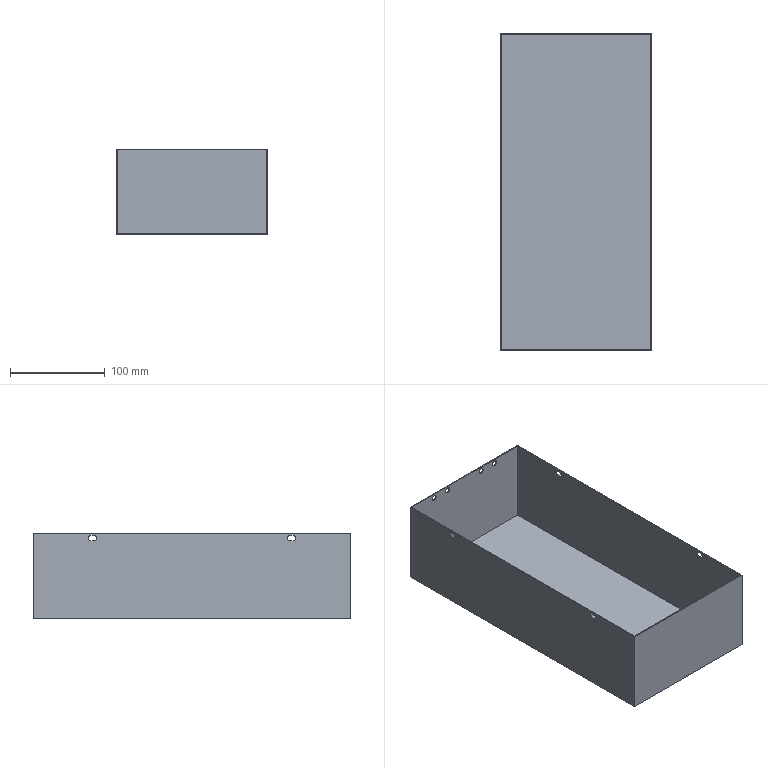Part | SolidWorks | features ICE 2, Extrusion 1, Shell 1 | 1 solid | 35 faces | box 160 x 335 x 90 mm | volume 168968 mm3 | plane 19 | cylinder 16 | commonest cylinder face diameters 5.6 x8 6 x8
STEP:
#1=CARTESIAN_POINT('',(-45.,166.3,88.));
#2=VERTEX_POINT('',#1);
#3=CARTESIAN_POINT('',(-45.,166.3,82.));
#4=VERTEX_POINT('',#3);
#5=CARTESIAN_POINT('',(-45.,166.3,85.));
#6=DIRECTION('',(0.,-1.,0.));
#7=DIRECTION('',(0.,0.,-1.));
#8=AXIS2_PLACEMENT_3D('',#5,#6,#7);
#9=CIRCLE('',#8,3.);
#10=EDGE_CURVE('',#2,#4,#9,.T.);
#11=ORIENTED_EDGE('',*,*,#10,.T.);
#12=CARTESIAN_POINT('',(-45.,167.5,82.));
#13=VERTEX_POINT('',#12);
#14=CARTESIAN_POINT('',(-45.,157.5,82.));
#15=DIRECTION('',(0.,1.,0.));
#16=VECTOR('',#15,1000.);
#17=LINE('',#14,#16);
#18=EDGE_CURVE('',#4,#13,#17,.T.);
#19=ORIENTED_EDGE('',*,*,#18,.T.);
#20=CARTESIAN_POINT('',(-45.,167.5,88.));
#21=VERTEX_POINT('',#20);
#22=CARTESIAN_POINT('',(-45.,167.5,85.));
#23=DIRECTION('',(0.,1.,0.));
#24=DIRECTION('',(0.,0.,1.));
#25=AXIS2_PLACEMENT_3D('',#22,#23,#24);
#26=CIRCLE('',#25,3.);
#27=EDGE_CURVE('',#13,#21,#26,.T.);
#28=ORIENTED_EDGE('',*,*,#27,.T.);
#29=CARTESIAN_POINT('',(-45.,157.5,88.));
#30=DIRECTION('',(0.,1.,0.));
#31=VECTOR('',#30,1000.);
#32=LINE('',#29,#31);
#33=EDGE_CURVE('',#2,#21,#32,.T.);
#34=ORIENTED_EDGE('',*,*,#33,.F.);
#35=EDGE_LOOP('',(#11,#19,#28,#34));
#36=FACE_OUTER_BOUND('',#35,.T.);
#37=CARTESIAN_POINT('',(-45.,157.5,85.));
#38=DIRECTION('',(0.,1.,0.));
#39=DIRECTION('',(0.,0.,1.));
#40=AXIS2_PLACEMENT_3D('',#37,#38,#39);
#41=CYLINDRICAL_SURFACE('',#40,3.);
#42=ADVANCED_FACE('',(#36),#41,.F.);
#43=CARTESIAN_POINT('',(-25.,166.3,88.));
#44=VERTEX_POINT('',#43);
#45=CARTESIAN_POINT('',(-25.,166.3,82.));
#46=VERTEX_POINT('',#45);
#47=CARTESIAN_POINT('',(-25.,166.3,85.));
#48=DIRECTION('',(0.,-1.,0.));
#49=DIRECTION('',(0.,0.,-1.));
#50=AXIS2_PLACEMENT_3D('',#47,#48,#49);
#51=CIRCLE('',#50,3.);
#52=EDGE_CURVE('',#44,#46,#51,.T.);
#53=ORIENTED_EDGE('',*,*,#52,.T.);
#54=CARTESIAN_POINT('',(-25.,167.5,82.));
#55=VERTEX_POINT('',#54);
#56=CARTESIAN_POINT('',(-25.,157.5,82.));
#57=DIRECTION('',(0.,1.,0.));
#58=VECTOR('',#57,1000.);
#59=LINE('',#56,#58);
#60=EDGE_CURVE('',#46,#55,#59,.T.);
#61=ORIENTED_EDGE('',*,*,#60,.T.);
#62=CARTESIAN_POINT('',(-25.,167.5,88.));
#63=VERTEX_POINT('',#62);
#64=CARTESIAN_POINT('',(-25.,167.5,85.));
#65=DIRECTION('',(0.,1.,0.));
#66=DIRECTION('',(0.,0.,1.));
#67=AXIS2_PLACEMENT_3D('',#64,#65,#66);
#68=CIRCLE('',#67,3.);
#69=EDGE_CURVE('',#55,#63,#68,.T.);
#70=ORIENTED_EDGE('',*,*,#69,.T.);
#71=CARTESIAN_POINT('',(-25.,157.5,88.));
#72=DIRECTION('',(0.,1.,0.));
#73=VECTOR('',#72,1000.);
#74=LINE('',#71,#73);
#75=EDGE_CURVE('',#44,#63,#74,.T.);
#76=ORIENTED_EDGE('',*,*,#75,.F.);
#77=EDGE_LOOP('',(#53,#61,#70,#76));
#78=FACE_OUTER_BOUND('',#77,.T.);
#79=CARTESIAN_POINT('',(-25.,157.5,85.));
#80=DIRECTION('',(0.,1.,0.));
#81=DIRECTION('',(0.,0.,1.));
#82=AXIS2_PLACEMENT_3D('',#79,#80,#81);
#83=CYLINDRICAL_SURFACE('',#82,3.);
#84=ADVANCED_FACE('',(#78),#83,.F.);
#85=CARTESIAN_POINT('',(25.,166.3,88.));
#86=VERTEX_POINT('',#85);
#87=CARTESIAN_POINT('',(25.,166.3,82.));
#88=VERTEX_POINT('',#87);
#89=CARTESIAN_POINT('',(25.,166.3,85.));
#90=DIRECTION('',(0.,-1.,0.));
#91=DIRECTION('',(0.,0.,-1.));
#92=AXIS2_PLACEMENT_3D('',#89,#90,#91);
#93=CIRCLE('',#92,3.);
#94=EDGE_CURVE('',#86,#88,#93,.T.);
#95=ORIENTED_EDGE('',*,*,#94,.T.);
#96=CARTESIAN_POINT('',(25.,167.5,82.));
#97=VERTEX_POINT('',#96);
#98=CARTESIAN_POINT('',(25.,157.5,82.));
#99=DIRECTION('',(0.,1.,0.));
#100=VECTOR('',#99,1000.);
#101=LINE('',#98,#100);
#102=EDGE_CURVE('',#88,#97,#101,.T.);
#103=ORIENTED_EDGE('',*,*,#102,.T.);
#104=CARTESIAN_POINT('',(25.,167.5,88.));
#105=VERTEX_POINT('',#104);
#106=CARTESIAN_POINT('',(25.,167.5,85.));
#107=DIRECTION('',(0.,1.,0.));
#108=DIRECTION('',(0.,0.,1.));
#109=AXIS2_PLACEMENT_3D('',#106,#107,#108);
#110=CIRCLE('',#109,3.);
#111=EDGE_CURVE('',#97,#105,#110,.T.);
#112=ORIENTED_EDGE('',*,*,#111,.T.);
#113=CARTESIAN_POINT('',(25.,157.5,88.));
#114=DIRECTION('',(0.,1.,0.));
#115=VECTOR('',#114,1000.);
#116=LINE('',#113,#115);
#117=EDGE_CURVE('',#86,#105,#116,.T.);
#118=ORIENTED_EDGE('',*,*,#117,.F.);
#119=EDGE_LOOP('',(#95,#103,#112,#118));
#120=FACE_OUTER_BOUND('',#119,.T.);
#121=CARTESIAN_POINT('',(25.,157.5,85.));
#122=DIRECTION('',(0.,1.,0.));
#123=DIRECTION('',(0.,0.,1.));
#124=AXIS2_PLACEMENT_3D('',#121,#122,#123);
#125=CYLINDRICAL_SURFACE('',#124,3.);
#126=ADVANCED_FACE('',(#120),#125,.F.);
#127=CARTESIAN_POINT('',(45.,166.3,88.));
#128=VERTEX_POINT('',#127);
#129=CARTESIAN_POINT('',(45.,166.3,82.));
#130=VERTEX_POINT('',#129);
#131=CARTESIAN_POINT('',(45.,166.3,85.));
#132=DIRECTION('',(0.,-1.,0.));
#133=DIRECTION('',(0.,0.,-1.));
#134=AXIS2_PLACEMENT_3D('',#131,#132,#133);
#135=CIRCLE('',#134,3.);
#136=EDGE_CURVE('',#128,#130,#135,.T.);
#137=ORIENTED_EDGE('',*,*,#136,.T.);
#138=CARTESIAN_POINT('',(45.,167.5,82.));
#139=VERTEX_POINT('',#138);
#140=CARTESIAN_POINT('',(45.,157.5,82.));
#141=DIRECTION('',(0.,1.,0.));
#142=VECTOR('',#141,1000.);
#143=LINE('',#140,#142);
#144=EDGE_CURVE('',#130,#139,#143,.T.);
#145=ORIENTED_EDGE('',*,*,#144,.T.);
#146=CARTESIAN_POINT('',(45.,167.5,88.));
#147=VERTEX_POINT('',#146);
#148=CARTESIAN_POINT('',(45.,167.5,85.));
#149=DIRECTION('',(0.,1.,0.));
#150=DIRECTION('',(0.,0.,1.));
#151=AXIS2_PLACEMENT_3D('',#148,#149,#150);
#152=CIRCLE('',#151,3.);
#153=EDGE_CURVE('',#139,#147,#152,.T.);
#154=ORIENTED_EDGE('',*,*,#153,.T.);
#155=CARTESIAN_POINT('',(45.,157.5,88.));
#156=DIRECTION('',(0.,1.,0.));
#157=VECTOR('',#156,1000.);
#158=LINE('',#155,#157);
#159=EDGE_CURVE('',#128,#147,#158,.T.);
#160=ORIENTED_EDGE('',*,*,#159,.F.);
#161=EDGE_LOOP('',(#137,#145,#154,#160));
#162=FACE_OUTER_BOUND('',#161,.T.);
#163=CARTESIAN_POINT('',(45.,157.5,85.));
#164=DIRECTION('',(0.,1.,0.));
#165=DIRECTION('',(0.,0.,1.));
#166=AXIS2_PLACEMENT_3D('',#163,#164,#165);
#167=CYLINDRICAL_SURFACE('',#166,3.);
#168=ADVANCED_FACE('',(#162),#167,.F.);
#169=CARTESIAN_POINT('',(80.,-167.5,90.));
#170=VERTEX_POINT('',#169);
#171=CARTESIAN_POINT('',(80.,167.5,90.));
#172=VERTEX_POINT('',#171);
#173=CARTESIAN_POINT('',(80.,-167.5,90.));
#174=DIRECTION('',(0.,1.,0.));
#175=VECTOR('',#174,1000.);
#176=LINE('',#173,#175);
#177=EDGE_CURVE('',#170,#172,#176,.T.);
#178=ORIENTED_EDGE('',*,*,#177,.T.);
#179=CARTESIAN_POINT('',(-80.,167.5,90.));
#180=VERTEX_POINT('',#179);
#181=CARTESIAN_POINT('',(-80.,167.5,90.));
#182=DIRECTION('',(-1.,0.,0.));
#183=VECTOR('',#182,1000.);
#184=LINE('',#181,#183);
#185=EDGE_CURVE('',#172,#180,#184,.T.);
#186=ORIENTED_EDGE('',*,*,#185,.T.);
#187=CARTESIAN_POINT('',(-80.,-167.5,90.));
#188=VERTEX_POINT('',#187);
#189=CARTESIAN_POINT('',(-80.,-167.5,90.));
#190=DIRECTION('',(0.,-1.,0.));
#191=VECTOR('',#190,1000.);
#192=LINE('',#189,#191);
#193=EDGE_CURVE('',#180,#188,#192,.T.);
#194=ORIENTED_EDGE('',*,*,#193,.T.);
#195=CARTESIAN_POINT('',(-80.,-167.5,90.));
#196=DIRECTION('',(1.,0.,0.));
#197=VECTOR('',#196,1000.);
#198=LINE('',#195,#197);
#199=EDGE_CURVE('',#188,#170,#198,.T.);
#200=ORIENTED_EDGE('',*,*,#199,.T.);
#201=EDGE_LOOP('',(#178,#186,#194,#200));
#202=FACE_OUTER_BOUND('',#201,.T.);
#203=CARTESIAN_POINT('',(78.8,-166.3,90.));
#204=VERTEX_POINT('',#203);
#205=CARTESIAN_POINT('',(78.8,166.3,90.));
#206=VERTEX_POINT('',#205);
#207=CARTESIAN_POINT('',(78.8,0.,90.));
#208=DIRECTION('',(0.,1.,0.));
#209=VECTOR('',#208,1000.);
#210=LINE('',#207,#209);
#211=EDGE_CURVE('',#204,#206,#210,.T.);
#212=ORIENTED_EDGE('',*,*,#211,.F.);
#213=CARTESIAN_POINT('',(-78.8,-166.3,90.));
#214=VERTEX_POINT('',#213);
#215=CARTESIAN_POINT('',(0.,-166.3,90.));
#216=DIRECTION('',(1.,0.,0.));
#217=VECTOR('',#216,1000.);
#218=LINE('',#215,#217);
#219=EDGE_CURVE('',#214,#204,#218,.T.);
#220=ORIENTED_EDGE('',*,*,#219,.F.);
#221=CARTESIAN_POINT('',(-78.8,166.3,90.));
#222=VERTEX_POINT('',#221);
#223=CARTESIAN_POINT('',(-78.8,0.,90.));
#224=DIRECTION('',(0.,-1.,0.));
#225=VECTOR('',#224,1000.);
#226=LINE('',#223,#225);
#227=EDGE_CURVE('',#222,#214,#226,.T.);
#228=ORIENTED_EDGE('',*,*,#227,.F.);
#229=CARTESIAN_POINT('',(0.,166.3,90.));
#230=DIRECTION('',(-1.,0.,0.));
#231=VECTOR('',#230,1000.);
#232=LINE('',#229,#231);
#233=EDGE_CURVE('',#206,#222,#232,.T.);
#234=ORIENTED_EDGE('',*,*,#233,.F.);
#235=EDGE_LOOP('',(#212,#220,#228,#234));
#236=FACE_BOUND('',#235,.T.);
#237=CARTESIAN_POINT('',(0.,0.,90.));
#238=DIRECTION('',(0.,0.,-1.));
#239=DIRECTION('',(-1.,0.,0.));
#240=AXIS2_PLACEMENT_3D('',#237,#238,#239);
#241=PLANE('',#240);
#242=ADVANCED_FACE('',(#202,#236),#241,.F.);
#243=CARTESIAN_POINT('',(80.,103.5,87.8));
#244=VERTEX_POINT('',#243);
#245=CARTESIAN_POINT('',(80.,106.5,87.8));
#246=VERTEX_POINT('',#245);
#247=CARTESIAN_POINT('',(80.,106.5,87.8));
#248=DIRECTION('',(0.,1.,0.));
#249=VECTOR('',#248,1000.);
#250=LINE('',#247,#249);
#251=EDGE_CURVE('',#244,#246,#250,.T.);
#252=ORIENTED_EDGE('',*,*,#251,.T.);
#253=CARTESIAN_POINT('',(80.,106.5,82.2));
#254=VERTEX_POINT('',#253);
#255=CARTESIAN_POINT('',(80.,106.5,85.));
#256=DIRECTION('',(-1.,0.,0.));
#257=DIRECTION('',(0.,0.,1.));
#258=AXIS2_PLACEMENT_3D('',#255,#256,#257);
#259=CIRCLE('',#258,2.8);
#260=EDGE_CURVE('',#246,#254,#259,.T.);
#261=ORIENTED_EDGE('',*,*,#260,.T.);
#262=CARTESIAN_POINT('',(80.,103.5,82.2));
#263=VERTEX_POINT('',#262);
#264=CARTESIAN_POINT('',(80.,106.5,82.2));
#265=DIRECTION('',(0.,-1.,0.));
#266=VECTOR('',#265,1000.);
#267=LINE('',#264,#266);
#268=EDGE_CURVE('',#254,#263,#267,.T.);
#269=ORIENTED_EDGE('',*,*,#268,.T.);
#270=CARTESIAN_POINT('',(80.,103.5,85.));
#271=DIRECTION('',(-1.,0.,0.));
#272=DIRECTION('',(0.,0.,1.));
#273=AXIS2_PLACEMENT_3D('',#270,#271,#272);
#274=CIRCLE('',#273,2.8);
#275=EDGE_CURVE('',#263,#244,#274,.T.);
#276=ORIENTED_EDGE('',*,*,#275,.T.);
#277=EDGE_LOOP('',(#252,#261,#269,#276));
#278=FACE_BOUND('',#277,.T.);
#279=CARTESIAN_POINT('',(80.,-103.5,82.2));
#280=VERTEX_POINT('',#279);
#281=CARTESIAN_POINT('',(80.,-106.5,82.2));
#282=VERTEX_POINT('',#281);
#283=CARTESIAN_POINT('',(80.,-106.5,82.2));
#284=DIRECTION('',(0.,-1.,0.));
#285=VECTOR('',#284,1000.);
#286=LINE('',#283,#285);
#287=EDGE_CURVE('',#280,#282,#286,.T.);
#288=ORIENTED_EDGE('',*,*,#287,.T.);
#289=CARTESIAN_POINT('',(80.,-106.5,87.8));
#290=VERTEX_POINT('',#289);
#291=CARTESIAN_POINT('',(80.,-106.5,85.));
#292=DIRECTION('',(-1.,0.,0.));
#293=DIRECTION('',(0.,0.,-1.));
#294=AXIS2_PLACEMENT_3D('',#291,#292,#293);
#295=CIRCLE('',#294,2.8);
#296=EDGE_CURVE('',#282,#290,#295,.T.);
#297=ORIENTED_EDGE('',*,*,#296,.T.);
#298=CARTESIAN_POINT('',(80.,-103.5,87.8));
#299=VERTEX_POINT('',#298);
#300=CARTESIAN_POINT('',(80.,-106.5,87.8));
#301=DIRECTION('',(0.,1.,0.));
#302=VECTOR('',#301,1000.);
#303=LINE('',#300,#302);
#304=EDGE_CURVE('',#290,#299,#303,.T.);
#305=ORIENTED_EDGE('',*,*,#304,.T.);
#306=CARTESIAN_POINT('',(80.,-103.5,85.));
#307=DIRECTION('',(-1.,0.,0.));
#308=DIRECTION('',(0.,0.,-1.));
#309=AXIS2_PLACEMENT_3D('',#306,#307,#308);
#310=CIRCLE('',#309,2.8);
#311=EDGE_CURVE('',#299,#280,#310,.T.);
#312=ORIENTED_EDGE('',*,*,#311,.T.);
#313=EDGE_LOOP('',(#288,#297,#305,#312));
#314=FACE_BOUND('',#313,.T.);
#315=CARTESIAN_POINT('',(80.,-167.5,0.));
#316=VERTEX_POINT('',#315);
#317=CARTESIAN_POINT('',(80.,167.5,0.));
#318=VERTEX_POINT('',#317);
#319=CARTESIAN_POINT('',(80.,-167.5,0.));
#320=DIRECTION('',(0.,1.,0.));
#321=VECTOR('',#320,1000.);
#322=LINE('',#319,#321);
#323=EDGE_CURVE('',#316,#318,#322,.T.);
#324=ORIENTED_EDGE('',*,*,#323,.T.);
#325=CARTESIAN_POINT('',(80.,167.5,90.));
#326=DIRECTION('',(0.,0.,-1.));
#327=VECTOR('',#326,1000.);
#328=LINE('',#325,#327);
#329=EDGE_CURVE('',#172,#318,#328,.T.);
#330=ORIENTED_EDGE('',*,*,#329,.F.);
#331=ORIENTED_EDGE('',*,*,#177,.F.);
#332=CARTESIAN_POINT('',(80.,-167.5,90.));
#333=DIRECTION('',(0.,0.,-1.));
#334=VECTOR('',#333,1000.);
#335=LINE('',#332,#334);
#336=EDGE_CURVE('',#170,#316,#335,.T.);
#337=ORIENTED_EDGE('',*,*,#336,.T.);
#338=EDGE_LOOP('',(#324,#330,#331,#337));
#339=FACE_OUTER_BOUND('',#338,.T.);
#340=CARTESIAN_POINT('',(80.,-167.5,90.));
#341=DIRECTION('',(-1.,0.,0.));
#342=DIRECTION('',(0.,0.,1.));
#343=AXIS2_PLACEMENT_3D('',#340,#341,#342);
#344=PLANE('',#343);
#345=ADVANCED_FACE('',(#278,#314,#339),#344,.F.);
#346=CARTESIAN_POINT('',(-45.,167.5,85.));
#347=DIRECTION('',(0.,1.,0.));
#348=DIRECTION('',(0.,0.,1.));
#349=AXIS2_PLACEMENT_3D('',#346,#347,#348);
#350=CIRCLE('',#349,3.);
#351=EDGE_CURVE('',#21,#13,#350,.T.);
#352=ORIENTED_EDGE('',*,*,#351,.F.);
#353=ORIENTED_EDGE('',*,*,#27,.F.);
#354=EDGE_LOOP('',(#352,#353));
#355=FACE_BOUND('',#354,.T.);
#356=CARTESIAN_POINT('',(-25.,167.5,85.));
#357=DIRECTION('',(0.,1.,0.));
#358=DIRECTION('',(0.,0.,1.));
#359=AXIS2_PLACEMENT_3D('',#356,#357,#358);
#360=CIRCLE('',#359,3.);
#361=EDGE_CURVE('',#63,#55,#360,.T.);
#362=ORIENTED_EDGE('',*,*,#361,.F.);
#363=ORIENTED_EDGE('',*,*,#69,.F.);
#364=EDGE_LOOP('',(#362,#363));
#365=FACE_BOUND('',#364,.T.);
#366=CARTESIAN_POINT('',(25.,167.5,85.));
#367=DIRECTION('',(0.,1.,0.));
#368=DIRECTION('',(0.,0.,1.));
#369=AXIS2_PLACEMENT_3D('',#366,#367,#368);
#370=CIRCLE('',#369,3.);
#371=EDGE_CURVE('',#105,#97,#370,.T.);
#372=ORIENTED_EDGE('',*,*,#371,.F.);
#373=ORIENTED_EDGE('',*,*,#111,.F.);
#374=EDGE_LOOP('',(#372,#373));
#375=FACE_BOUND('',#374,.T.);
#376=CARTESIAN_POINT('',(45.,167.5,85.));
#377=DIRECTION('',(0.,1.,0.));
#378=DIRECTION('',(0.,0.,1.));
#379=AXIS2_PLACEMENT_3D('',#376,#377,#378);
#380=CIRCLE('',#379,3.);
#381=EDGE_CURVE('',#147,#139,#380,.T.);
#382=ORIENTED_EDGE('',*,*,#381,.F.);
#383=ORIENTED_EDGE('',*,*,#153,.F.);
#384=EDGE_LOOP('',(#382,#383));
#385=FACE_BOUND('',#384,.T.);
#386=CARTESIAN_POINT('',(-80.,167.5,0.));
#387=VERTEX_POINT('',#386);
#388=CARTESIAN_POINT('',(-80.,167.5,0.));
#389=DIRECTION('',(-1.,0.,0.));
#390=VECTOR('',#389,1000.);
#391=LINE('',#388,#390);
#392=EDGE_CURVE('',#318,#387,#391,.T.);
#393=ORIENTED_EDGE('',*,*,#392,.T.);
#394=CARTESIAN_POINT('',(-80.,167.5,90.));
#395=DIRECTION('',(0.,0.,-1.));
#396=VECTOR('',#395,1000.);
#397=LINE('',#394,#396);
#398=EDGE_CURVE('',#180,#387,#397,.T.);
#399=ORIENTED_EDGE('',*,*,#398,.F.);
#400=ORIENTED_EDGE('',*,*,#185,.F.);
#401=ORIENTED_EDGE('',*,*,#329,.T.);
#402=EDGE_LOOP('',(#393,#399,#400,#401));
#403=FACE_OUTER_BOUND('',#402,.T.);
#404=CARTESIAN_POINT('',(-80.,167.5,90.));
#405=DIRECTION('',(0.,-1.,0.));
#406=DIRECTION('',(0.,0.,-1.));
#407=AXIS2_PLACEMENT_3D('',#404,#405,#406);
#408=PLANE('',#407);
#409=ADVANCED_FACE('',(#355,#365,#375,#385,#403),#408,.F.);
#410=CARTESIAN_POINT('',(-80.,106.5,82.2));
#411=VERTEX_POINT('',#410);
#412=CARTESIAN_POINT('',(-80.,103.5,82.2));
#413=VERTEX_POINT('',#412);
#414=CARTESIAN_POINT('',(-80.,106.5,82.2));
#415=DIRECTION('',(0.,-1.,0.));
#416=VECTOR('',#415,1000.);
#417=LINE('',#414,#416);
#418=EDGE_CURVE('',#411,#413,#417,.T.);
#419=ORIENTED_EDGE('',*,*,#418,.F.);
#420=CARTESIAN_POINT('',(-80.,106.5,87.8));
#421=VERTEX_POINT('',#420);
#422=CARTESIAN_POINT('',(-80.,106.5,85.));
#423=DIRECTION('',(-1.,0.,0.));
#424=DIRECTION('',(0.,0.,1.));
#425=AXIS2_PLACEMENT_3D('',#422,#423,#424);
#426=CIRCLE('',#425,2.8);
#427=EDGE_CURVE('',#421,#411,#426,.T.);
#428=ORIENTED_EDGE('',*,*,#427,.F.);
#429=CARTESIAN_POINT('',(-80.,103.5,87.8));
#430=VERTEX_POINT('',#429);
#431=CARTESIAN_POINT('',(-80.,106.5,87.8));
#432=DIRECTION('',(0.,1.,0.));
#433=VECTOR('',#432,1000.);
#434=LINE('',#431,#433);
#435=EDGE_CURVE('',#430,#421,#434,.T.);
#436=ORIENTED_EDGE('',*,*,#435,.F.);
#437=CARTESIAN_POINT('',(-80.,103.5,85.));
#438=DIRECTION('',(-1.,0.,0.));
#439=DIRECTION('',(0.,0.,1.));
#440=AXIS2_PLACEMENT_3D('',#437,#438,#439);
#441=CIRCLE('',#440,2.8);
#442=EDGE_CURVE('',#413,#430,#441,.T.);
#443=ORIENTED_EDGE('',*,*,#442,.F.);
#444=EDGE_LOOP('',(#419,#428,#436,#443));
#445=FACE_BOUND('',#444,.T.);
#446=CARTESIAN_POINT('',(-80.,-106.5,87.8));
#447=VERTEX_POINT('',#446);
#448=CARTESIAN_POINT('',(-80.,-103.5,87.8));
#449=VERTEX_POINT('',#448);
#450=CARTESIAN_POINT('',(-80.,-106.5,87.8));
#451=DIRECTION('',(0.,1.,0.));
#452=VECTOR('',#451,1000.);
#453=LINE('',#450,#452);
#454=EDGE_CURVE('',#447,#449,#453,.T.);
#455=ORIENTED_EDGE('',*,*,#454,.F.);
#456=CARTESIAN_POINT('',(-80.,-106.5,82.2));
#457=VERTEX_POINT('',#456);
#458=CARTESIAN_POINT('',(-80.,-106.5,85.));
#459=DIRECTION('',(-1.,0.,0.));
#460=DIRECTION('',(0.,0.,-1.));
#461=AXIS2_PLACEMENT_3D('',#458,#459,#460);
#462=CIRCLE('',#461,2.8);
#463=EDGE_CURVE('',#457,#447,#462,.T.);
#464=ORIENTED_EDGE('',*,*,#463,.F.);
#465=CARTESIAN_POINT('',(-80.,-103.5,82.2));
#466=VERTEX_POINT('',#465);
#467=CARTESIAN_POINT('',(-80.,-106.5,82.2));
#468=DIRECTION('',(0.,-1.,0.));
#469=VECTOR('',#468,1000.);
#470=LINE('',#467,#469);
#471=EDGE_CURVE('',#466,#457,#470,.T.);
#472=ORIENTED_EDGE('',*,*,#471,.F.);
#473=CARTESIAN_POINT('',(-80.,-103.5,85.));
#474=DIRECTION('',(-1.,0.,0.));
#475=DIRECTION('',(0.,0.,-1.));
#476=AXIS2_PLACEMENT_3D('',#473,#474,#475);
#477=CIRCLE('',#476,2.8);
#478=EDGE_CURVE('',#449,#466,#477,.T.);
#479=ORIENTED_EDGE('',*,*,#478,.F.);
#480=EDGE_LOOP('',(#455,#464,#472,#479));
#481=FACE_BOUND('',#480,.T.);
#482=CARTESIAN_POINT('',(-80.,-167.5,0.));
#483=VERTEX_POINT('',#482);
#484=CARTESIAN_POINT('',(-80.,-167.5,0.));
#485=DIRECTION('',(0.,-1.,0.));
#486=VECTOR('',#485,1000.);
#487=LINE('',#484,#486);
#488=EDGE_CURVE('',#387,#483,#487,.T.);
#489=ORIENTED_EDGE('',*,*,#488,.T.);
#490=CARTESIAN_POINT('',(-80.,-167.5,90.));
#491=DIRECTION('',(0.,0.,-1.));
#492=VECTOR('',#491,1000.);
#493=LINE('',#490,#492);
#494=EDGE_CURVE('',#188,#483,#493,.T.);
#495=ORIENTED_EDGE('',*,*,#494,.F.);
#496=ORIENTED_EDGE('',*,*,#193,.F.);
#497=ORIENTED_EDGE('',*,*,#398,.T.);
#498=EDGE_LOOP('',(#489,#495,#496,#497));
#499=FACE_OUTER_BOUND('',#498,.T.);
#500=CARTESIAN_POINT('',(-80.,-167.5,90.));
#501=DIRECTION('',(1.,0.,0.));
#502=DIRECTION('',(0.,0.,-1.));
#503=AXIS2_PLACEMENT_3D('',#500,#501,#502);
#504=PLANE('',#503);
#505=ADVANCED_FACE('',(#445,#481,#499),#504,.F.);
#506=CARTESIAN_POINT('',(-80.,-167.5,0.));
#507=DIRECTION('',(1.,0.,0.));
#508=VECTOR('',#507,1000.);
#509=LINE('',#506,#508);
#510=EDGE_CURVE('',#483,#316,#509,.T.);
#511=ORIENTED_EDGE('',*,*,#510,.T.);
#512=ORIENTED_EDGE('',*,*,#336,.F.);
#513=ORIENTED_EDGE('',*,*,#199,.F.);
#514=ORIENTED_EDGE('',*,*,#494,.T.);
#515=EDGE_LOOP('',(#511,#512,#513,#514));
#516=FACE_OUTER_BOUND('',#515,.T.);
#517=CARTESIAN_POINT('',(-80.,-167.5,90.));
#518=DIRECTION('',(0.,1.,0.));
#519=DIRECTION('',(0.,0.,1.));
#520=AXIS2_PLACEMENT_3D('',#517,#518,#519);
#521=PLANE('',#520);
#522=ADVANCED_FACE('',(#516),#521,.F.);
#523=ORIENTED_EDGE('',*,*,#323,.F.);
#524=ORIENTED_EDGE('',*,*,#510,.F.);
#525=ORIENTED_EDGE('',*,*,#488,.F.);
#526=ORIENTED_EDGE('',*,*,#392,.F.);
#527=EDGE_LOOP('',(#523,#524,#525,#526));
#528=FACE_OUTER_BOUND('',#527,.T.);
#529=CARTESIAN_POINT('',(0.,0.,0.));
#530=DIRECTION('',(0.,0.,-1.));
#531=DIRECTION('',(-1.,0.,0.));
#532=AXIS2_PLACEMENT_3D('',#529,#530,#531);
#533=PLANE('',#532);
#534=ADVANCED_FACE('',(#528),#533,.T.);
#535=CARTESIAN_POINT('',(78.8,106.5,87.8));
#536=VERTEX_POINT('',#535);
#537=CARTESIAN_POINT('',(78.8,106.5,82.2));
#538=VERTEX_POINT('',#537);
#539=CARTESIAN_POINT('',(78.8,106.5,85.));
#540=DIRECTION('',(-1.,0.,0.));
#541=DIRECTION('',(0.,0.,1.));
#542=AXIS2_PLACEMENT_3D('',#539,#540,#541);
#543=CIRCLE('',#542,2.8);
#544=EDGE_CURVE('',#536,#538,#543,.T.);
#545=ORIENTED_EDGE('',*,*,#544,.F.);
#546=CARTESIAN_POINT('',(78.8,103.5,87.8));
#547=VERTEX_POINT('',#546);
#548=CARTESIAN_POINT('',(78.8,-167.5,87.8));
#549=DIRECTION('',(0.,1.,0.));
#550=VECTOR('',#549,1000.);
#551=LINE('',#548,#550);
#552=EDGE_CURVE('',#547,#536,#551,.T.);
#553=ORIENTED_EDGE('',*,*,#552,.F.);
#554=CARTESIAN_POINT('',(78.8,103.5,82.2));
#555=VERTEX_POINT('',#554);
#556=CARTESIAN_POINT('',(78.8,103.5,85.));
#557=DIRECTION('',(-1.,0.,0.));
#558=DIRECTION('',(0.,0.,1.));
#559=AXIS2_PLACEMENT_3D('',#556,#557,#558);
#560=CIRCLE('',#559,2.8);
#561=EDGE_CURVE('',#555,#547,#560,.T.);
#562=ORIENTED_EDGE('',*,*,#561,.F.);
#563=CARTESIAN_POINT('',(78.8,-167.5,82.2));
#564=DIRECTION('',(0.,-1.,0.));
#565=VECTOR('',#564,1000.);
#566=LINE('',#563,#565);
#567=EDGE_CURVE('',#538,#555,#566,.T.);
#568=ORIENTED_EDGE('',*,*,#567,.F.);
#569=EDGE_LOOP('',(#545,#553,#562,#568));
#570=FACE_BOUND('',#569,.T.);
#571=CARTESIAN_POINT('',(78.8,-106.5,82.2));
#572=VERTEX_POINT('',#571);
#573=CARTESIAN_POINT('',(78.8,-106.5,87.8));
#574=VERTEX_POINT('',#573);
#575=CARTESIAN_POINT('',(78.8,-106.5,85.));
#576=DIRECTION('',(-1.,0.,0.));
#577=DIRECTION('',(0.,0.,1.));
#578=AXIS2_PLACEMENT_3D('',#575,#576,#577);
#579=CIRCLE('',#578,2.8);
#580=EDGE_CURVE('',#572,#574,#579,.T.);
#581=ORIENTED_EDGE('',*,*,#580,.F.);
#582=CARTESIAN_POINT('',(78.8,-103.5,82.2));
#583=VERTEX_POINT('',#582);
#584=CARTESIAN_POINT('',(78.8,-167.5,82.2));
#585=DIRECTION('',(0.,-1.,0.));
#586=VECTOR('',#585,1000.);
#587=LINE('',#584,#586);
#588=EDGE_CURVE('',#583,#572,#587,.T.);
#589=ORIENTED_EDGE('',*,*,#588,.F.);
#590=CARTESIAN_POINT('',(78.8,-103.5,87.8));
#591=VERTEX_POINT('',#590);
#592=CARTESIAN_POINT('',(78.8,-103.5,85.));
#593=DIRECTION('',(-1.,0.,0.));
#594=DIRECTION('',(0.,0.,1.));
#595=AXIS2_PLACEMENT_3D('',#592,#593,#594);
#596=CIRCLE('',#595,2.8);
#597=EDGE_CURVE('',#591,#583,#596,.T.);
#598=ORIENTED_EDGE('',*,*,#597,.F.);
#599=CARTESIAN_POINT('',(78.8,-167.5,87.8));
#600=DIRECTION('',(0.,1.,0.));
#601=VECTOR('',#600,1000.);
#602=LINE('',#599,#601);
#603=EDGE_CURVE('',#574,#591,#602,.T.);
#604=ORIENTED_EDGE('',*,*,#603,.F.);
#605=EDGE_LOOP('',(#581,#589,#598,#604));
#606=FACE_BOUND('',#605,.T.);
#607=CARTESIAN_POINT('',(78.8,-166.3,1.2));
#608=VERTEX_POINT('',#607);
#609=CARTESIAN_POINT('',(78.8,166.3,1.2));
#610=VERTEX_POINT('',#609);
#611=CARTESIAN_POINT('',(78.8,0.,1.2));
#612=DIRECTION('',(0.,1.,0.));
#613=VECTOR('',#612,1000.);
#614=LINE('',#611,#613);
#615=EDGE_CURVE('',#608,#610,#614,.T.);
#616=ORIENTED_EDGE('',*,*,#615,.F.);
#617=CARTESIAN_POINT('',(78.8,-166.3,90.));
#618=DIRECTION('',(0.,0.,-1.));
#619=VECTOR('',#618,1000.);
#620=LINE('',#617,#619);
#621=EDGE_CURVE('',#204,#608,#620,.T.);
#622=ORIENTED_EDGE('',*,*,#621,.F.);
#623=ORIENTED_EDGE('',*,*,#211,.T.);
#624=CARTESIAN_POINT('',(78.8,166.3,90.));
#625=DIRECTION('',(0.,0.,-1.));
#626=VECTOR('',#625,1000.);
#627=LINE('',#624,#626);
#628=EDGE_CURVE('',#206,#610,#627,.T.);
#629=ORIENTED_EDGE('',*,*,#628,.T.);
#630=EDGE_LOOP('',(#616,#622,#623,#629));
#631=FACE_OUTER_BOUND('',#630,.T.);
#632=CARTESIAN_POINT('',(78.8,-167.5,90.));
#633=DIRECTION('',(-1.,0.,0.));
#634=DIRECTION('',(0.,0.,1.));
#635=AXIS2_PLACEMENT_3D('',#632,#633,#634);
#636=PLANE('',#635);
#637=ADVANCED_FACE('',(#570,#606,#631),#636,.T.);
#638=ORIENTED_EDGE('',*,*,#10,.F.);
#639=CARTESIAN_POINT('',(-45.,166.3,85.));
#640=DIRECTION('',(0.,-1.,0.));
#641=DIRECTION('',(0.,0.,-1.));
#642=AXIS2_PLACEMENT_3D('',#639,#640,#641);
#643=CIRCLE('',#642,3.);
#644=EDGE_CURVE('',#4,#2,#643,.T.);
#645=ORIENTED_EDGE('',*,*,#644,.F.);
#646=EDGE_LOOP('',(#638,#645));
#647=FACE_BOUND('',#646,.T.);
#648=ORIENTED_EDGE('',*,*,#52,.F.);
#649=CARTESIAN_POINT('',(-25.,166.3,85.));
#650=DIRECTION('',(0.,-1.,0.));
#651=DIRECTION('',(0.,0.,-1.));
#652=AXIS2_PLACEMENT_3D('',#649,#650,#651);
#653=CIRCLE('',#652,3.);
#654=EDGE_CURVE('',#46,#44,#653,.T.);
#655=ORIENTED_EDGE('',*,*,#654,.F.);
#656=EDGE_LOOP('',(#648,#655));
#657=FACE_BOUND('',#656,.T.);
#658=ORIENTED_EDGE('',*,*,#94,.F.);
#659=CARTESIAN_POINT('',(25.,166.3,85.));
#660=DIRECTION('',(0.,-1.,0.));
#661=DIRECTION('',(0.,0.,-1.));
#662=AXIS2_PLACEMENT_3D('',#659,#660,#661);
#663=CIRCLE('',#662,3.);
#664=EDGE_CURVE('',#88,#86,#663,.T.);
#665=ORIENTED_EDGE('',*,*,#664,.F.);
#666=EDGE_LOOP('',(#658,#665));
#667=FACE_BOUND('',#666,.T.);
#668=ORIENTED_EDGE('',*,*,#136,.F.);
#669=CARTESIAN_POINT('',(45.,166.3,85.));
#670=DIRECTION('',(0.,-1.,0.));
#671=DIRECTION('',(0.,0.,-1.));
#672=AXIS2_PLACEMENT_3D('',#669,#670,#671);
#673=CIRCLE('',#672,3.);
#674=EDGE_CURVE('',#130,#128,#673,.T.);
#675=ORIENTED_EDGE('',*,*,#674,.F.);
#676=EDGE_LOOP('',(#668,#675));
#677=FACE_BOUND('',#676,.T.);
#678=CARTESIAN_POINT('',(-78.8,166.3,1.2));
#679=VERTEX_POINT('',#678);
#680=CARTESIAN_POINT('',(0.,166.3,1.2));
#681=DIRECTION('',(-1.,0.,0.));
#682=VECTOR('',#681,1000.);
#683=LINE('',#680,#682);
#684=EDGE_CURVE('',#610,#679,#683,.T.);
#685=ORIENTED_EDGE('',*,*,#684,.F.);
#686=ORIENTED_EDGE('',*,*,#628,.F.);
#687=ORIENTED_EDGE('',*,*,#233,.T.);
#688=CARTESIAN_POINT('',(-78.8,166.3,90.));
#689=DIRECTION('',(0.,0.,-1.));
#690=VECTOR('',#689,1000.);
#691=LINE('',#688,#690);
#692=EDGE_CURVE('',#222,#679,#691,.T.);
#693=ORIENTED_EDGE('',*,*,#692,.T.);
#694=EDGE_LOOP('',(#685,#686,#687,#693));
#695=FACE_OUTER_BOUND('',#694,.T.);
#696=CARTESIAN_POINT('',(-80.,166.3,90.));
#697=DIRECTION('',(0.,-1.,0.));
#698=DIRECTION('',(0.,0.,-1.));
#699=AXIS2_PLACEMENT_3D('',#696,#697,#698);
#700=PLANE('',#699);
#701=ADVANCED_FACE('',(#647,#657,#667,#677,#695),#700,.T.);
#702=CARTESIAN_POINT('',(-78.8,106.5,82.2));
#703=VERTEX_POINT('',#702);
#704=CARTESIAN_POINT('',(-78.8,106.5,87.8));
#705=VERTEX_POINT('',#704);
#706=CARTESIAN_POINT('',(-78.8,106.5,85.));
#707=DIRECTION('',(1.,0.,0.));
#708=DIRECTION('',(0.,0.,-1.));
#709=AXIS2_PLACEMENT_3D('',#706,#707,#708);
#710=CIRCLE('',#709,2.8);
#711=EDGE_CURVE('',#703,#705,#710,.T.);
#712=ORIENTED_EDGE('',*,*,#711,.F.);
#713=CARTESIAN_POINT('',(-78.8,103.5,82.2));
#714=VERTEX_POINT('',#713);
#715=CARTESIAN_POINT('',(-78.8,-167.5,82.2));
#716=DIRECTION('',(0.,1.,0.));
#717=VECTOR('',#716,1000.);
#718=LINE('',#715,#717);
#719=EDGE_CURVE('',#714,#703,#718,.T.);
#720=ORIENTED_EDGE('',*,*,#719,.F.);
#721=CARTESIAN_POINT('',(-78.8,103.5,87.8));
#722=VERTEX_POINT('',#721);
#723=CARTESIAN_POINT('',(-78.8,103.5,85.));
#724=DIRECTION('',(1.,0.,0.));
#725=DIRECTION('',(0.,0.,-1.));
#726=AXIS2_PLACEMENT_3D('',#723,#724,#725);
#727=CIRCLE('',#726,2.8);
#728=EDGE_CURVE('',#722,#714,#727,.T.);
#729=ORIENTED_EDGE('',*,*,#728,.F.);
#730=CARTESIAN_POINT('',(-78.8,-167.5,87.8));
#731=DIRECTION('',(0.,-1.,0.));
#732=VECTOR('',#731,1000.);
#733=LINE('',#730,#732);
#734=EDGE_CURVE('',#705,#722,#733,.T.);
#735=ORIENTED_EDGE('',*,*,#734,.F.);
#736=EDGE_LOOP('',(#712,#720,#729,#735));
#737=FACE_BOUND('',#736,.T.);
#738=CARTESIAN_POINT('',(-78.8,-106.5,87.8));
#739=VERTEX_POINT('',#738);
#740=CARTESIAN_POINT('',(-78.8,-106.5,82.2));
#741=VERTEX_POINT('',#740);
#742=CARTESIAN_POINT('',(-78.8,-106.5,85.));
#743=DIRECTION('',(1.,0.,0.));
#744=DIRECTION('',(0.,0.,-1.));
#745=AXIS2_PLACEMENT_3D('',#742,#743,#744);
#746=CIRCLE('',#745,2.8);
#747=EDGE_CURVE('',#739,#741,#746,.T.);
#748=ORIENTED_EDGE('',*,*,#747,.F.);
#749=CARTESIAN_POINT('',(-78.8,-103.5,87.8));
#750=VERTEX_POINT('',#749);
#751=CARTESIAN_POINT('',(-78.8,-167.5,87.8));
#752=DIRECTION('',(0.,-1.,0.));
#753=VECTOR('',#752,1000.);
#754=LINE('',#751,#753);
#755=EDGE_CURVE('',#750,#739,#754,.T.);
#756=ORIENTED_EDGE('',*,*,#755,.F.);
#757=CARTESIAN_POINT('',(-78.8,-103.5,82.2));
#758=VERTEX_POINT('',#757);
#759=CARTESIAN_POINT('',(-78.8,-103.5,85.));
#760=DIRECTION('',(1.,0.,0.));
#761=DIRECTION('',(0.,0.,-1.));
#762=AXIS2_PLACEMENT_3D('',#759,#760,#761);
#763=CIRCLE('',#762,2.8);
#764=EDGE_CURVE('',#758,#750,#763,.T.);
#765=ORIENTED_EDGE('',*,*,#764,.F.);
#766=CARTESIAN_POINT('',(-78.8,-167.5,82.2));
#767=DIRECTION('',(0.,1.,0.));
#768=VECTOR('',#767,1000.);
#769=LINE('',#766,#768);
#770=EDGE_CURVE('',#741,#758,#769,.T.);
#771=ORIENTED_EDGE('',*,*,#770,.F.);
#772=EDGE_LOOP('',(#748,#756,#765,#771));
#773=FACE_BOUND('',#772,.T.);
#774=CARTESIAN_POINT('',(-78.8,-166.3,1.2));
#775=VERTEX_POINT('',#774);
#776=CARTESIAN_POINT('',(-78.8,0.,1.2));
#777=DIRECTION('',(0.,-1.,0.));
#778=VECTOR('',#777,1000.);
#779=LINE('',#776,#778);
#780=EDGE_CURVE('',#679,#775,#779,.T.);
#781=ORIENTED_EDGE('',*,*,#780,.F.);
#782=ORIENTED_EDGE('',*,*,#692,.F.);
#783=ORIENTED_EDGE('',*,*,#227,.T.);
#784=CARTESIAN_POINT('',(-78.8,-166.3,90.));
#785=DIRECTION('',(0.,0.,-1.));
#786=VECTOR('',#785,1000.);
#787=LINE('',#784,#786);
#788=EDGE_CURVE('',#214,#775,#787,.T.);
#789=ORIENTED_EDGE('',*,*,#788,.T.);
#790=EDGE_LOOP('',(#781,#782,#783,#789));
#791=FACE_OUTER_BOUND('',#790,.T.);
#792=CARTESIAN_POINT('',(-78.8,-167.5,90.));
#793=DIRECTION('',(1.,0.,0.));
#794=DIRECTION('',(0.,0.,-1.));
#795=AXIS2_PLACEMENT_3D('',#792,#793,#794);
#796=PLANE('',#795);
#797=ADVANCED_FACE('',(#737,#773,#791),#796,.T.);
#798=CARTESIAN_POINT('',(0.,-166.3,1.2));
#799=DIRECTION('',(1.,0.,0.));
#800=VECTOR('',#799,1000.);
#801=LINE('',#798,#800);
#802=EDGE_CURVE('',#775,#608,#801,.T.);
#803=ORIENTED_EDGE('',*,*,#802,.F.);
#804=ORIENTED_EDGE('',*,*,#788,.F.);
#805=ORIENTED_EDGE('',*,*,#219,.T.);
#806=ORIENTED_EDGE('',*,*,#621,.T.);
#807=EDGE_LOOP('',(#803,#804,#805,#806));
#808=FACE_OUTER_BOUND('',#807,.T.);
#809=CARTESIAN_POINT('',(-80.,-166.3,90.));
#810=DIRECTION('',(0.,1.,0.));
#811=DIRECTION('',(0.,0.,1.));
#812=AXIS2_PLACEMENT_3D('',#809,#810,#811);
#813=PLANE('',#812);
#814=ADVANCED_FACE('',(#808),#813,.T.);
#815=ORIENTED_EDGE('',*,*,#615,.T.);
#816=ORIENTED_EDGE('',*,*,#684,.T.);
#817=ORIENTED_EDGE('',*,*,#780,.T.);
#818=ORIENTED_EDGE('',*,*,#802,.T.);
#819=EDGE_LOOP('',(#815,#816,#817,#818));
#820=FACE_OUTER_BOUND('',#819,.T.);
#821=CARTESIAN_POINT('',(0.,0.,1.2));
#822=DIRECTION('',(0.,0.,-1.));
#823=DIRECTION('',(-1.,0.,0.));
#824=AXIS2_PLACEMENT_3D('',#821,#822,#823);
#825=PLANE('',#824);
#826=ADVANCED_FACE('',(#820),#825,.F.);
#827=ORIENTED_EDGE('',*,*,#144,.F.);
#828=ORIENTED_EDGE('',*,*,#674,.T.);
#829=ORIENTED_EDGE('',*,*,#159,.T.);
#830=ORIENTED_EDGE('',*,*,#381,.T.);
#831=EDGE_LOOP('',(#827,#828,#829,#830));
#832=FACE_OUTER_BOUND('',#831,.T.);
#833=CARTESIAN_POINT('',(45.,157.5,85.));
#834=DIRECTION('',(0.,1.,0.));
#835=DIRECTION('',(0.,0.,1.));
#836=AXIS2_PLACEMENT_3D('',#833,#834,#835);
#837=CYLINDRICAL_SURFACE('',#836,3.);
#838=ADVANCED_FACE('',(#832),#837,.F.);
#839=ORIENTED_EDGE('',*,*,#102,.F.);
#840=ORIENTED_EDGE('',*,*,#664,.T.);
#841=ORIENTED_EDGE('',*,*,#117,.T.);
#842=ORIENTED_EDGE('',*,*,#371,.T.);
#843=EDGE_LOOP('',(#839,#840,#841,#842));
#844=FACE_OUTER_BOUND('',#843,.T.);
#845=CARTESIAN_POINT('',(25.,157.5,85.));
#846=DIRECTION('',(0.,1.,0.));
#847=DIRECTION('',(0.,0.,1.));
#848=AXIS2_PLACEMENT_3D('',#845,#846,#847);
#849=CYLINDRICAL_SURFACE('',#848,3.);
#850=ADVANCED_FACE('',(#844),#849,.F.);
#851=ORIENTED_EDGE('',*,*,#60,.F.);
#852=ORIENTED_EDGE('',*,*,#654,.T.);
#853=ORIENTED_EDGE('',*,*,#75,.T.);
#854=ORIENTED_EDGE('',*,*,#361,.T.);
#855=EDGE_LOOP('',(#851,#852,#853,#854));
#856=FACE_OUTER_BOUND('',#855,.T.);
#857=CARTESIAN_POINT('',(-25.,157.5,85.));
#858=DIRECTION('',(0.,1.,0.));
#859=DIRECTION('',(0.,0.,1.));
#860=AXIS2_PLACEMENT_3D('',#857,#858,#859);
#861=CYLINDRICAL_SURFACE('',#860,3.);
#862=ADVANCED_FACE('',(#856),#861,.F.);
#863=ORIENTED_EDGE('',*,*,#18,.F.);
#864=ORIENTED_EDGE('',*,*,#644,.T.);
#865=ORIENTED_EDGE('',*,*,#33,.T.);
#866=ORIENTED_EDGE('',*,*,#351,.T.);
#867=EDGE_LOOP('',(#863,#864,#865,#866));
#868=FACE_OUTER_BOUND('',#867,.T.);
#869=CARTESIAN_POINT('',(-45.,157.5,85.));
#870=DIRECTION('',(0.,1.,0.));
#871=DIRECTION('',(0.,0.,1.));
#872=AXIS2_PLACEMENT_3D('',#869,#870,#871);
#873=CYLINDRICAL_SURFACE('',#872,3.);
#874=ADVANCED_FACE('',(#868),#873,.F.);
#875=ORIENTED_EDGE('',*,*,#755,.T.);
#876=CARTESIAN_POINT('',(80.,-106.5,87.8));
#877=DIRECTION('',(-1.,0.,0.));
#878=VECTOR('',#877,1000.);
#879=LINE('',#876,#878);
#880=EDGE_CURVE('',#739,#447,#879,.T.);
#881=ORIENTED_EDGE('',*,*,#880,.T.);
#882=ORIENTED_EDGE('',*,*,#454,.T.);
#883=CARTESIAN_POINT('',(80.,-103.5,87.8));
#884=DIRECTION('',(-1.,0.,0.));
#885=VECTOR('',#884,1000.);
#886=LINE('',#883,#885);
#887=EDGE_CURVE('',#750,#449,#886,.T.);
#888=ORIENTED_EDGE('',*,*,#887,.F.);
#889=EDGE_LOOP('',(#875,#881,#882,#888));
#890=FACE_OUTER_BOUND('',#889,.T.);
#891=CARTESIAN_POINT('',(80.,-106.5,87.8));
#892=DIRECTION('',(0.,0.,1.));
#893=DIRECTION('',(1.,0.,0.));
#894=AXIS2_PLACEMENT_3D('',#891,#892,#893);
#895=PLANE('',#894);
#896=ADVANCED_FACE('',(#890),#895,.F.);
#897=ORIENTED_EDGE('',*,*,#764,.T.);
#898=ORIENTED_EDGE('',*,*,#887,.T.);
#899=ORIENTED_EDGE('',*,*,#478,.T.);
#900=CARTESIAN_POINT('',(80.,-103.5,82.2));
#901=DIRECTION('',(-1.,0.,0.));
#902=VECTOR('',#901,1000.);
#903=LINE('',#900,#902);
#904=EDGE_CURVE('',#758,#466,#903,.T.);
#905=ORIENTED_EDGE('',*,*,#904,.F.);
#906=EDGE_LOOP('',(#897,#898,#899,#905));
#907=FACE_OUTER_BOUND('',#906,.T.);
#908=CARTESIAN_POINT('',(80.,-103.5,85.));
#909=DIRECTION('',(-1.,0.,0.));
#910=DIRECTION('',(0.,0.,1.));
#911=AXIS2_PLACEMENT_3D('',#908,#909,#910);
#912=CYLINDRICAL_SURFACE('',#911,2.8);
#913=ADVANCED_FACE('',(#907),#912,.F.);
#914=ORIENTED_EDGE('',*,*,#770,.T.);
#915=ORIENTED_EDGE('',*,*,#904,.T.);
#916=ORIENTED_EDGE('',*,*,#471,.T.);
#917=CARTESIAN_POINT('',(80.,-106.5,82.2));
#918=DIRECTION('',(-1.,0.,0.));
#919=VECTOR('',#918,1000.);
#920=LINE('',#917,#919);
#921=EDGE_CURVE('',#741,#457,#920,.T.);
#922=ORIENTED_EDGE('',*,*,#921,.F.);
#923=EDGE_LOOP('',(#914,#915,#916,#922));
#924=FACE_OUTER_BOUND('',#923,.T.);
#925=CARTESIAN_POINT('',(80.,-106.5,82.2));
#926=DIRECTION('',(0.,0.,-1.));
#927=DIRECTION('',(-1.,0.,0.));
#928=AXIS2_PLACEMENT_3D('',#925,#926,#927);
#929=PLANE('',#928);
#930=ADVANCED_FACE('',(#924),#929,.F.);
#931=ORIENTED_EDGE('',*,*,#747,.T.);
#932=ORIENTED_EDGE('',*,*,#921,.T.);
#933=ORIENTED_EDGE('',*,*,#463,.T.);
#934=ORIENTED_EDGE('',*,*,#880,.F.);
#935=EDGE_LOOP('',(#931,#932,#933,#934));
#936=FACE_OUTER_BOUND('',#935,.T.);
#937=CARTESIAN_POINT('',(80.,-106.5,85.));
#938=DIRECTION('',(-1.,0.,0.));
#939=DIRECTION('',(0.,0.,1.));
#940=AXIS2_PLACEMENT_3D('',#937,#938,#939);
#941=CYLINDRICAL_SURFACE('',#940,2.8);
#942=ADVANCED_FACE('',(#936),#941,.F.);
#943=ORIENTED_EDGE('',*,*,#719,.T.);
#944=CARTESIAN_POINT('',(80.,106.5,82.2));
#945=DIRECTION('',(-1.,0.,0.));
#946=VECTOR('',#945,1000.);
#947=LINE('',#944,#946);
#948=EDGE_CURVE('',#703,#411,#947,.T.);
#949=ORIENTED_EDGE('',*,*,#948,.T.);
#950=ORIENTED_EDGE('',*,*,#418,.T.);
#951=CARTESIAN_POINT('',(80.,103.5,82.2));
#952=DIRECTION('',(-1.,0.,0.));
#953=VECTOR('',#952,1000.);
#954=LINE('',#951,#953);
#955=EDGE_CURVE('',#714,#413,#954,.T.);
#956=ORIENTED_EDGE('',*,*,#955,.F.);
#957=EDGE_LOOP('',(#943,#949,#950,#956));
#958=FACE_OUTER_BOUND('',#957,.T.);
#959=CARTESIAN_POINT('',(80.,106.5,82.2));
#960=DIRECTION('',(0.,0.,-1.));
#961=DIRECTION('',(-1.,0.,0.));
#962=AXIS2_PLACEMENT_3D('',#959,#960,#961);
#963=PLANE('',#962);
#964=ADVANCED_FACE('',(#958),#963,.F.);
#965=ORIENTED_EDGE('',*,*,#728,.T.);
#966=ORIENTED_EDGE('',*,*,#955,.T.);
#967=ORIENTED_EDGE('',*,*,#442,.T.);
#968=CARTESIAN_POINT('',(80.,103.5,87.8));
#969=DIRECTION('',(-1.,0.,0.));
#970=VECTOR('',#969,1000.);
#971=LINE('',#968,#970);
#972=EDGE_CURVE('',#722,#430,#971,.T.);
#973=ORIENTED_EDGE('',*,*,#972,.F.);
#974=EDGE_LOOP('',(#965,#966,#967,#973));
#975=FACE_OUTER_BOUND('',#974,.T.);
#976=CARTESIAN_POINT('',(80.,103.5,85.));
#977=DIRECTION('',(-1.,0.,0.));
#978=DIRECTION('',(0.,0.,1.));
#979=AXIS2_PLACEMENT_3D('',#976,#977,#978);
#980=CYLINDRICAL_SURFACE('',#979,2.8);
#981=ADVANCED_FACE('',(#975),#980,.F.);
#982=ORIENTED_EDGE('',*,*,#734,.T.);
#983=ORIENTED_EDGE('',*,*,#972,.T.);
#984=ORIENTED_EDGE('',*,*,#435,.T.);
#985=CARTESIAN_POINT('',(80.,106.5,87.8));
#986=DIRECTION('',(-1.,0.,0.));
#987=VECTOR('',#986,1000.);
#988=LINE('',#985,#987);
#989=EDGE_CURVE('',#705,#421,#988,.T.);
#990=ORIENTED_EDGE('',*,*,#989,.F.);
#991=EDGE_LOOP('',(#982,#983,#984,#990));
#992=FACE_OUTER_BOUND('',#991,.T.);
#993=CARTESIAN_POINT('',(80.,106.5,87.8));
#994=DIRECTION('',(0.,0.,1.));
#995=DIRECTION('',(1.,0.,0.));
#996=AXIS2_PLACEMENT_3D('',#993,#994,#995);
#997=PLANE('',#996);
#998=ADVANCED_FACE('',(#992),#997,.F.);
#999=ORIENTED_EDGE('',*,*,#711,.T.);
#1000=ORIENTED_EDGE('',*,*,#989,.T.);
#1001=ORIENTED_EDGE('',*,*,#427,.T.);
#1002=ORIENTED_EDGE('',*,*,#948,.F.);
#1003=EDGE_LOOP('',(#999,#1000,#1001,#1002));
#1004=FACE_OUTER_BOUND('',#1003,.T.);
#1005=CARTESIAN_POINT('',(80.,106.5,85.));
#1006=DIRECTION('',(-1.,0.,0.));
#1007=DIRECTION('',(0.,0.,1.));
#1008=AXIS2_PLACEMENT_3D('',#1005,#1006,#1007);
#1009=CYLINDRICAL_SURFACE('',#1008,2.8);
#1010=ADVANCED_FACE('',(#1004),#1009,.F.);
#1011=ORIENTED_EDGE('',*,*,#580,.T.);
#1012=CARTESIAN_POINT('',(80.,-106.5,87.8));
#1013=DIRECTION('',(-1.,0.,0.));
#1014=VECTOR('',#1013,1000.);
#1015=LINE('',#1012,#1014);
#1016=EDGE_CURVE('',#290,#574,#1015,.T.);
#1017=ORIENTED_EDGE('',*,*,#1016,.F.);
#1018=ORIENTED_EDGE('',*,*,#296,.F.);
#1019=CARTESIAN_POINT('',(80.,-106.5,82.2));
#1020=DIRECTION('',(-1.,0.,0.));
#1021=VECTOR('',#1020,1000.);
#1022=LINE('',#1019,#1021);
#1023=EDGE_CURVE('',#282,#572,#1022,.T.);
#1024=ORIENTED_EDGE('',*,*,#1023,.T.);
#1025=EDGE_LOOP('',(#1011,#1017,#1018,#1024));
#1026=FACE_OUTER_BOUND('',#1025,.T.);
#1027=CARTESIAN_POINT('',(80.,-106.5,85.));
#1028=DIRECTION('',(-1.,0.,0.));
#1029=DIRECTION('',(0.,0.,1.));
#1030=AXIS2_PLACEMENT_3D('',#1027,#1028,#1029);
#1031=CYLINDRICAL_SURFACE('',#1030,2.8);
#1032=ADVANCED_FACE('',(#1026),#1031,.F.);
#1033=ORIENTED_EDGE('',*,*,#588,.T.);
#1034=ORIENTED_EDGE('',*,*,#1023,.F.);
#1035=ORIENTED_EDGE('',*,*,#287,.F.);
#1036=CARTESIAN_POINT('',(80.,-103.5,82.2));
#1037=DIRECTION('',(-1.,0.,0.));
#1038=VECTOR('',#1037,1000.);
#1039=LINE('',#1036,#1038);
#1040=EDGE_CURVE('',#280,#583,#1039,.T.);
#1041=ORIENTED_EDGE('',*,*,#1040,.T.);
#1042=EDGE_LOOP('',(#1033,#1034,#1035,#1041));
#1043=FACE_OUTER_BOUND('',#1042,.T.);
#1044=CARTESIAN_POINT('',(80.,-106.5,82.2));
#1045=DIRECTION('',(0.,0.,-1.));
#1046=DIRECTION('',(-1.,0.,0.));
#1047=AXIS2_PLACEMENT_3D('',#1044,#1045,#1046);
#1048=PLANE('',#1047);
#1049=ADVANCED_FACE('',(#1043),#1048,.F.);
#1050=ORIENTED_EDGE('',*,*,#597,.T.);
#1051=ORIENTED_EDGE('',*,*,#1040,.F.);
#1052=ORIENTED_EDGE('',*,*,#311,.F.);
#1053=CARTESIAN_POINT('',(80.,-103.5,87.8));
#1054=DIRECTION('',(-1.,0.,0.));
#1055=VECTOR('',#1054,1000.);
#1056=LINE('',#1053,#1055);
#1057=EDGE_CURVE('',#299,#591,#1056,.T.);
#1058=ORIENTED_EDGE('',*,*,#1057,.T.);
#1059=EDGE_LOOP('',(#1050,#1051,#1052,#1058));
#1060=FACE_OUTER_BOUND('',#1059,.T.);
#1061=CARTESIAN_POINT('',(80.,-103.5,85.));
#1062=DIRECTION('',(-1.,0.,0.));
#1063=DIRECTION('',(0.,0.,1.));
#1064=AXIS2_PLACEMENT_3D('',#1061,#1062,#1063);
#1065=CYLINDRICAL_SURFACE('',#1064,2.8);
#1066=ADVANCED_FACE('',(#1060),#1065,.F.);
#1067=ORIENTED_EDGE('',*,*,#603,.T.);
#1068=ORIENTED_EDGE('',*,*,#1057,.F.);
#1069=ORIENTED_EDGE('',*,*,#304,.F.);
#1070=ORIENTED_EDGE('',*,*,#1016,.T.);
#1071=EDGE_LOOP('',(#1067,#1068,#1069,#1070));
#1072=FACE_OUTER_BOUND('',#1071,.T.);
#1073=CARTESIAN_POINT('',(80.,-106.5,87.8));
#1074=DIRECTION('',(0.,0.,1.));
#1075=DIRECTION('',(1.,0.,0.));
#1076=AXIS2_PLACEMENT_3D('',#1073,#1074,#1075);
#1077=PLANE('',#1076);
#1078=ADVANCED_FACE('',(#1072),#1077,.F.);
#1079=ORIENTED_EDGE('',*,*,#544,.T.);
#1080=CARTESIAN_POINT('',(80.,106.5,82.2));
#1081=DIRECTION('',(-1.,0.,0.));
#1082=VECTOR('',#1081,1000.);
#1083=LINE('',#1080,#1082);
#1084=EDGE_CURVE('',#254,#538,#1083,.T.);
#1085=ORIENTED_EDGE('',*,*,#1084,.F.);
#1086=ORIENTED_EDGE('',*,*,#260,.F.);
#1087=CARTESIAN_POINT('',(80.,106.5,87.8));
#1088=DIRECTION('',(-1.,0.,0.));
#1089=VECTOR('',#1088,1000.);
#1090=LINE('',#1087,#1089);
#1091=EDGE_CURVE('',#246,#536,#1090,.T.);
#1092=ORIENTED_EDGE('',*,*,#1091,.T.);
#1093=EDGE_LOOP('',(#1079,#1085,#1086,#1092));
#1094=FACE_OUTER_BOUND('',#1093,.T.);
#1095=CARTESIAN_POINT('',(80.,106.5,85.));
#1096=DIRECTION('',(-1.,0.,0.));
#1097=DIRECTION('',(0.,0.,1.));
#1098=AXIS2_PLACEMENT_3D('',#1095,#1096,#1097);
#1099=CYLINDRICAL_SURFACE('',#1098,2.8);
#1100=ADVANCED_FACE('',(#1094),#1099,.F.);
#1101=ORIENTED_EDGE('',*,*,#552,.T.);
#1102=ORIENTED_EDGE('',*,*,#1091,.F.);
#1103=ORIENTED_EDGE('',*,*,#251,.F.);
#1104=CARTESIAN_POINT('',(80.,103.5,87.8));
#1105=DIRECTION('',(-1.,0.,0.));
#1106=VECTOR('',#1105,1000.);
#1107=LINE('',#1104,#1106);
#1108=EDGE_CURVE('',#244,#547,#1107,.T.);
#1109=ORIENTED_EDGE('',*,*,#1108,.T.);
#1110=EDGE_LOOP('',(#1101,#1102,#1103,#1109));
#1111=FACE_OUTER_BOUND('',#1110,.T.);
#1112=CARTESIAN_POINT('',(80.,106.5,87.8));
#1113=DIRECTION('',(0.,0.,1.));
#1114=DIRECTION('',(1.,0.,0.));
#1115=AXIS2_PLACEMENT_3D('',#1112,#1113,#1114);
#1116=PLANE('',#1115);
#1117=ADVANCED_FACE('',(#1111),#1116,.F.);
#1118=ORIENTED_EDGE('',*,*,#561,.T.);
#1119=ORIENTED_EDGE('',*,*,#1108,.F.);
#1120=ORIENTED_EDGE('',*,*,#275,.F.);
#1121=CARTESIAN_POINT('',(80.,103.5,82.2));
#1122=DIRECTION('',(-1.,0.,0.));
#1123=VECTOR('',#1122,1000.);
#1124=LINE('',#1121,#1123);
#1125=EDGE_CURVE('',#263,#555,#1124,.T.);
#1126=ORIENTED_EDGE('',*,*,#1125,.T.);
#1127=EDGE_LOOP('',(#1118,#1119,#1120,#1126));
#1128=FACE_OUTER_BOUND('',#1127,.T.);
#1129=CARTESIAN_POINT('',(80.,103.5,85.));
#1130=DIRECTION('',(-1.,0.,0.));
#1131=DIRECTION('',(0.,0.,1.));
#1132=AXIS2_PLACEMENT_3D('',#1129,#1130,#1131);
#1133=CYLINDRICAL_SURFACE('',#1132,2.8);
#1134=ADVANCED_FACE('',(#1128),#1133,.F.);
#1135=ORIENTED_EDGE('',*,*,#567,.T.);
#1136=ORIENTED_EDGE('',*,*,#1125,.F.);
#1137=ORIENTED_EDGE('',*,*,#268,.F.);
#1138=ORIENTED_EDGE('',*,*,#1084,.T.);
#1139=EDGE_LOOP('',(#1135,#1136,#1137,#1138));
#1140=FACE_OUTER_BOUND('',#1139,.T.);
#1141=CARTESIAN_POINT('',(80.,106.5,82.2));
#1142=DIRECTION('',(0.,0.,-1.));
#1143=DIRECTION('',(-1.,0.,0.));
#1144=AXIS2_PLACEMENT_3D('',#1141,#1142,#1143);
#1145=PLANE('',#1144);
#1146=ADVANCED_FACE('',(#1140),#1145,.F.);
#1147=CLOSED_SHELL('',(#42,#84,#126,#168,#242,#345,#409,#505,#522,#534,#637,#701,#797,#814,#826,#838,#850,#862,#874,#896,#913,#930,#942,#964,#981,#998,#1010,#1032,#1049,#1066,#1078,#1100,#1117,#1134,#1146));
#1148=MANIFOLD_SOLID_BREP('',#1147);
#1149=CARTESIAN_POINT('',(0.,0.,0.));
#1150=DIRECTION('',(0.,0.,1.));
#1151=DIRECTION('',(1.,0.,0.));
#1152=AXIS2_PLACEMENT_3D('',#1149,#1150,#1151);
#1153=(LENGTH_UNIT()NAMED_UNIT(*)SI_UNIT(.MILLI.,.METRE.));
#1154=UNCERTAINTY_MEASURE_WITH_UNIT(LENGTH_MEASURE(0.00001),#1153,'','');
#1155=(NAMED_UNIT(*)PLANE_ANGLE_UNIT()SI_UNIT($,.RADIAN.));
#1156=(NAMED_UNIT(*)SI_UNIT($,.STERADIAN.)SOLID_ANGLE_UNIT());
#1157=(GEOMETRIC_REPRESENTATION_CONTEXT(3)GLOBAL_UNCERTAINTY_ASSIGNED_CONTEXT((#1154))GLOBAL_UNIT_ASSIGNED_CONTEXT((#1153,#1155,#1156))REPRESENTATION_CONTEXT('',''));
#1158=ADVANCED_BREP_SHAPE_REPRESENTATION('',(#1148,#1152),#1157);